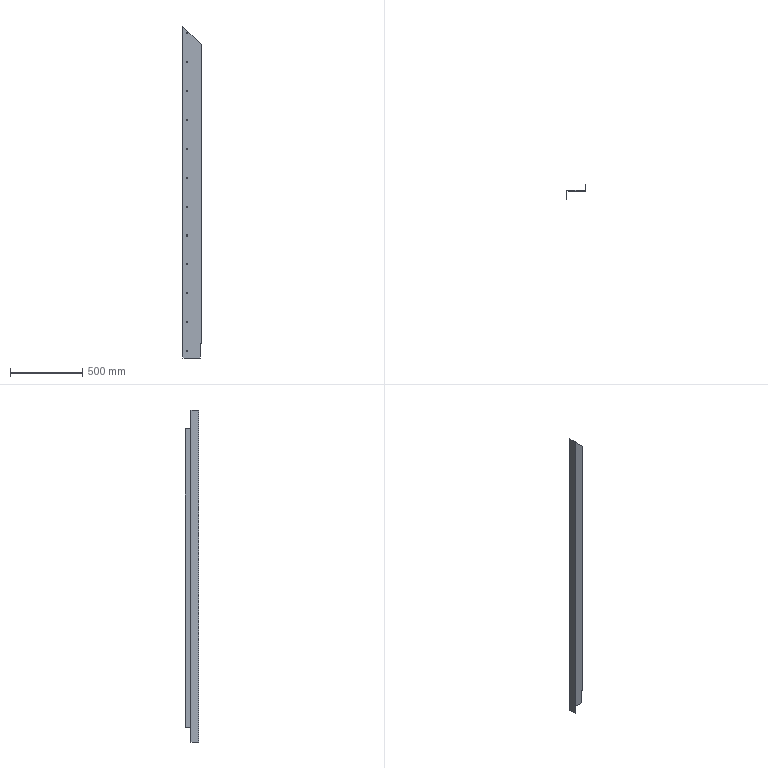Part | STEP file | TS-Z001-001 | 1 solid | 49 faces | box 131 x 95 x 2298 mm | volume 1471322 mm3 | cylinder 28 | plane 19 | spline 2 | commonest cylinder face diameters 8 x24 0.4 x2 6.4 x2